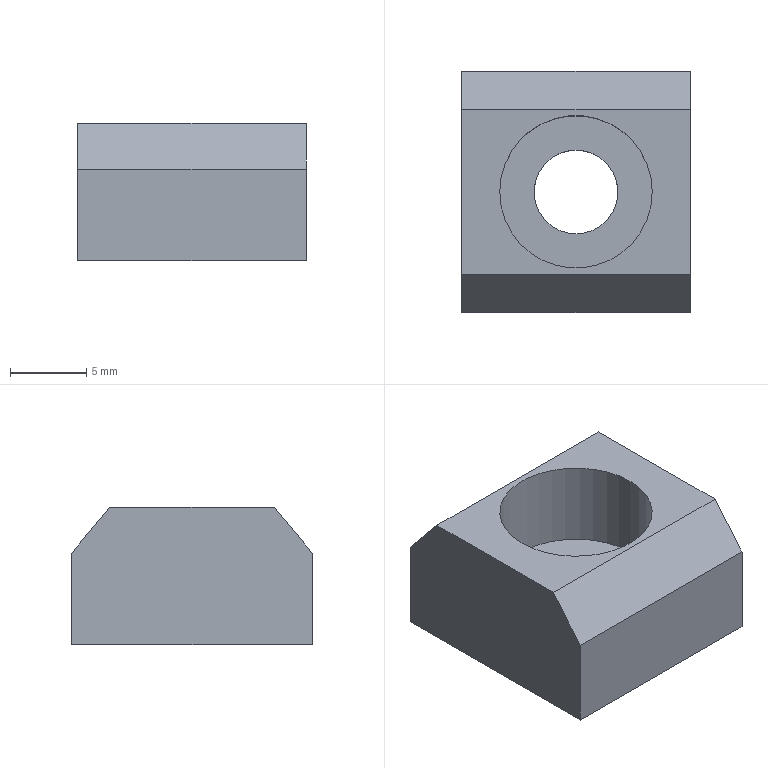Part | SolidWorks | features Extrusion 1, HoleWzd 1, ICE 1 | 1 solid | 13 faces | box 15 x 15.8 x 9 mm | volume 1494 mm3 | plane 9 | cylinder 4 | commonest cylinder face diameters 5.5 x2 10 x2
STEP:
#1=CARTESIAN_POINT('',(-5.,0.,-1.2));
#2=VERTEX_POINT('',#1);
#3=CARTESIAN_POINT('',(5.,0.,-1.2));
#4=VERTEX_POINT('',#3);
#5=CARTESIAN_POINT('',(0.,0.,-1.2));
#6=DIRECTION('',(0.,0.,1.));
#7=DIRECTION('',(1.,0.,0.));
#8=AXIS2_PLACEMENT_3D('',#5,#6,#7);
#9=CIRCLE('',#8,5.);
#10=EDGE_CURVE('',#2,#4,#9,.T.);
#11=ORIENTED_EDGE('',*,*,#10,.F.);
#12=CARTESIAN_POINT('',(-5.,0.,4.5));
#13=VERTEX_POINT('',#12);
#14=CARTESIAN_POINT('',(-5.,0.,4.5));
#15=DIRECTION('',(0.,0.,1.));
#16=VECTOR('',#15,1000.);
#17=LINE('',#14,#16);
#18=EDGE_CURVE('',#2,#13,#17,.T.);
#19=ORIENTED_EDGE('',*,*,#18,.T.);
#20=CARTESIAN_POINT('',(5.,0.,4.5));
#21=VERTEX_POINT('',#20);
#22=CARTESIAN_POINT('',(0.,0.,4.5));
#23=DIRECTION('',(0.,0.,1.));
#24=DIRECTION('',(1.,0.,0.));
#25=AXIS2_PLACEMENT_3D('',#22,#23,#24);
#26=CIRCLE('',#25,5.);
#27=EDGE_CURVE('',#13,#21,#26,.T.);
#28=ORIENTED_EDGE('',*,*,#27,.T.);
#29=CARTESIAN_POINT('',(5.,0.,4.5));
#30=DIRECTION('',(0.,0.,1.));
#31=VECTOR('',#30,1000.);
#32=LINE('',#29,#31);
#33=EDGE_CURVE('',#4,#21,#32,.T.);
#34=ORIENTED_EDGE('',*,*,#33,.F.);
#35=EDGE_LOOP('',(#11,#19,#28,#34));
#36=FACE_OUTER_BOUND('',#35,.T.);
#37=CARTESIAN_POINT('',(0.,0.,4.5));
#38=DIRECTION('',(0.,0.,1.));
#39=DIRECTION('',(1.,0.,0.));
#40=AXIS2_PLACEMENT_3D('',#37,#38,#39);
#41=CYLINDRICAL_SURFACE('',#40,5.);
#42=ADVANCED_FACE('',(#36),#41,.F.);
#43=CARTESIAN_POINT('',(-2.75,0.,-4.5));
#44=VERTEX_POINT('',#43);
#45=CARTESIAN_POINT('',(2.75,0.,-4.5));
#46=VERTEX_POINT('',#45);
#47=CARTESIAN_POINT('',(0.,0.,-4.5));
#48=DIRECTION('',(0.,0.,1.));
#49=DIRECTION('',(1.,0.,0.));
#50=AXIS2_PLACEMENT_3D('',#47,#48,#49);
#51=CIRCLE('',#50,2.75);
#52=EDGE_CURVE('',#44,#46,#51,.T.);
#53=ORIENTED_EDGE('',*,*,#52,.F.);
#54=CARTESIAN_POINT('',(-2.75,0.,-1.2));
#55=VERTEX_POINT('',#54);
#56=CARTESIAN_POINT('',(-2.75,0.,4.5));
#57=DIRECTION('',(0.,0.,1.));
#58=VECTOR('',#57,1000.);
#59=LINE('',#56,#58);
#60=EDGE_CURVE('',#44,#55,#59,.T.);
#61=ORIENTED_EDGE('',*,*,#60,.T.);
#62=CARTESIAN_POINT('',(2.75,0.,-1.2));
#63=VERTEX_POINT('',#62);
#64=CARTESIAN_POINT('',(0.,0.,-1.2));
#65=DIRECTION('',(0.,0.,1.));
#66=DIRECTION('',(1.,0.,0.));
#67=AXIS2_PLACEMENT_3D('',#64,#65,#66);
#68=CIRCLE('',#67,2.75);
#69=EDGE_CURVE('',#55,#63,#68,.T.);
#70=ORIENTED_EDGE('',*,*,#69,.T.);
#71=CARTESIAN_POINT('',(2.75,0.,4.5));
#72=DIRECTION('',(0.,0.,1.));
#73=VECTOR('',#72,1000.);
#74=LINE('',#71,#73);
#75=EDGE_CURVE('',#46,#63,#74,.T.);
#76=ORIENTED_EDGE('',*,*,#75,.F.);
#77=EDGE_LOOP('',(#53,#61,#70,#76));
#78=FACE_OUTER_BOUND('',#77,.T.);
#79=CARTESIAN_POINT('',(0.,0.,4.5));
#80=DIRECTION('',(0.,0.,1.));
#81=DIRECTION('',(1.,0.,0.));
#82=AXIS2_PLACEMENT_3D('',#79,#80,#81);
#83=CYLINDRICAL_SURFACE('',#82,2.75);
#84=ADVANCED_FACE('',(#78),#83,.F.);
#85=CARTESIAN_POINT('',(7.5,-5.4,4.5));
#86=VERTEX_POINT('',#85);
#87=CARTESIAN_POINT('',(7.5,5.4,4.5));
#88=VERTEX_POINT('',#87);
#89=CARTESIAN_POINT('',(7.5,7.9,4.5));
#90=DIRECTION('',(0.,1.,0.));
#91=VECTOR('',#90,1000.);
#92=LINE('',#89,#91);
#93=EDGE_CURVE('',#86,#88,#92,.T.);
#94=ORIENTED_EDGE('',*,*,#93,.F.);
#95=CARTESIAN_POINT('',(7.5,-7.9,1.5));
#96=VERTEX_POINT('',#95);
#97=CARTESIAN_POINT('',(7.5,-5.4,4.5));
#98=DIRECTION('',(0.,0.6402,0.7682));
#99=VECTOR('',#98,1000.);
#100=LINE('',#97,#99);
#101=EDGE_CURVE('',#96,#86,#100,.T.);
#102=ORIENTED_EDGE('',*,*,#101,.F.);
#103=CARTESIAN_POINT('',(7.5,-7.9,-4.5));
#104=VERTEX_POINT('',#103);
#105=CARTESIAN_POINT('',(7.5,-7.9,4.5));
#106=DIRECTION('',(0.,0.,-1.));
#107=VECTOR('',#106,1000.);
#108=LINE('',#105,#107);
#109=EDGE_CURVE('',#96,#104,#108,.T.);
#110=ORIENTED_EDGE('',*,*,#109,.T.);
#111=CARTESIAN_POINT('',(7.5,7.9,-4.5));
#112=VERTEX_POINT('',#111);
#113=CARTESIAN_POINT('',(7.5,7.9,-4.5));
#114=DIRECTION('',(0.,1.,0.));
#115=VECTOR('',#114,1000.);
#116=LINE('',#113,#115);
#117=EDGE_CURVE('',#104,#112,#116,.T.);
#118=ORIENTED_EDGE('',*,*,#117,.T.);
#119=CARTESIAN_POINT('',(7.5,7.9,1.5));
#120=VERTEX_POINT('',#119);
#121=CARTESIAN_POINT('',(7.5,7.9,4.5));
#122=DIRECTION('',(0.,0.,-1.));
#123=VECTOR('',#122,1000.);
#124=LINE('',#121,#123);
#125=EDGE_CURVE('',#120,#112,#124,.T.);
#126=ORIENTED_EDGE('',*,*,#125,.F.);
#127=CARTESIAN_POINT('',(7.5,7.9,1.5));
#128=DIRECTION('',(0.,0.6402,-0.7682));
#129=VECTOR('',#128,1000.);
#130=LINE('',#127,#129);
#131=EDGE_CURVE('',#88,#120,#130,.T.);
#132=ORIENTED_EDGE('',*,*,#131,.F.);
#133=EDGE_LOOP('',(#94,#102,#110,#118,#126,#132));
#134=FACE_OUTER_BOUND('',#133,.T.);
#135=CARTESIAN_POINT('',(7.5,7.9,4.5));
#136=DIRECTION('',(-1.,0.,0.));
#137=DIRECTION('',(0.,-1.,0.));
#138=AXIS2_PLACEMENT_3D('',#135,#136,#137);
#139=PLANE('',#138);
#140=ADVANCED_FACE('',(#134),#139,.F.);
#141=CARTESIAN_POINT('',(-7.5,7.9,1.5));
#142=VERTEX_POINT('',#141);
#143=CARTESIAN_POINT('',(-7.5,7.9,-4.5));
#144=VERTEX_POINT('',#143);
#145=CARTESIAN_POINT('',(-7.5,7.9,4.5));
#146=DIRECTION('',(0.,0.,-1.));
#147=VECTOR('',#146,1000.);
#148=LINE('',#145,#147);
#149=EDGE_CURVE('',#142,#144,#148,.T.);
#150=ORIENTED_EDGE('',*,*,#149,.F.);
#151=CARTESIAN_POINT('',(-7.5,7.9,1.5));
#152=DIRECTION('',(1.,0.,0.));
#153=VECTOR('',#152,1000.);
#154=LINE('',#151,#153);
#155=EDGE_CURVE('',#142,#120,#154,.T.);
#156=ORIENTED_EDGE('',*,*,#155,.T.);
#157=ORIENTED_EDGE('',*,*,#125,.T.);
#158=CARTESIAN_POINT('',(-7.5,7.9,-4.5));
#159=DIRECTION('',(-1.,0.,0.));
#160=VECTOR('',#159,1000.);
#161=LINE('',#158,#160);
#162=EDGE_CURVE('',#112,#144,#161,.T.);
#163=ORIENTED_EDGE('',*,*,#162,.T.);
#164=EDGE_LOOP('',(#150,#156,#157,#163));
#165=FACE_OUTER_BOUND('',#164,.T.);
#166=CARTESIAN_POINT('',(-7.5,7.9,4.5));
#167=DIRECTION('',(0.,-1.,0.));
#168=DIRECTION('',(0.,0.,-1.));
#169=AXIS2_PLACEMENT_3D('',#166,#167,#168);
#170=PLANE('',#169);
#171=ADVANCED_FACE('',(#165),#170,.F.);
#172=CARTESIAN_POINT('',(-7.5,-7.9,1.5));
#173=VERTEX_POINT('',#172);
#174=CARTESIAN_POINT('',(-7.5,-7.9,-4.5));
#175=VERTEX_POINT('',#174);
#176=CARTESIAN_POINT('',(-7.5,-7.9,4.5));
#177=DIRECTION('',(0.,0.,-1.));
#178=VECTOR('',#177,1000.);
#179=LINE('',#176,#178);
#180=EDGE_CURVE('',#173,#175,#179,.T.);
#181=ORIENTED_EDGE('',*,*,#180,.F.);
#182=CARTESIAN_POINT('',(-7.5,-5.4,4.5));
#183=VERTEX_POINT('',#182);
#184=CARTESIAN_POINT('',(-7.5,-5.4,4.5));
#185=DIRECTION('',(0.,0.6402,0.7682));
#186=VECTOR('',#185,1000.);
#187=LINE('',#184,#186);
#188=EDGE_CURVE('',#173,#183,#187,.T.);
#189=ORIENTED_EDGE('',*,*,#188,.T.);
#190=CARTESIAN_POINT('',(-7.5,5.4,4.5));
#191=VERTEX_POINT('',#190);
#192=CARTESIAN_POINT('',(-7.5,7.9,4.5));
#193=DIRECTION('',(0.,-1.,0.));
#194=VECTOR('',#193,1000.);
#195=LINE('',#192,#194);
#196=EDGE_CURVE('',#191,#183,#195,.T.);
#197=ORIENTED_EDGE('',*,*,#196,.F.);
#198=CARTESIAN_POINT('',(-7.5,7.9,1.5));
#199=DIRECTION('',(0.,0.6402,-0.7682));
#200=VECTOR('',#199,1000.);
#201=LINE('',#198,#200);
#202=EDGE_CURVE('',#191,#142,#201,.T.);
#203=ORIENTED_EDGE('',*,*,#202,.T.);
#204=ORIENTED_EDGE('',*,*,#149,.T.);
#205=CARTESIAN_POINT('',(-7.5,7.9,-4.5));
#206=DIRECTION('',(0.,-1.,0.));
#207=VECTOR('',#206,1000.);
#208=LINE('',#205,#207);
#209=EDGE_CURVE('',#144,#175,#208,.T.);
#210=ORIENTED_EDGE('',*,*,#209,.T.);
#211=EDGE_LOOP('',(#181,#189,#197,#203,#204,#210));
#212=FACE_OUTER_BOUND('',#211,.T.);
#213=CARTESIAN_POINT('',(-7.5,7.9,4.5));
#214=DIRECTION('',(1.,0.,0.));
#215=DIRECTION('',(0.,1.,0.));
#216=AXIS2_PLACEMENT_3D('',#213,#214,#215);
#217=PLANE('',#216);
#218=ADVANCED_FACE('',(#212),#217,.F.);
#219=ORIENTED_EDGE('',*,*,#109,.F.);
#220=CARTESIAN_POINT('',(-7.5,-7.9,1.5));
#221=DIRECTION('',(1.,0.,0.));
#222=VECTOR('',#221,1000.);
#223=LINE('',#220,#222);
#224=EDGE_CURVE('',#173,#96,#223,.T.);
#225=ORIENTED_EDGE('',*,*,#224,.F.);
#226=ORIENTED_EDGE('',*,*,#180,.T.);
#227=CARTESIAN_POINT('',(-7.5,-7.9,-4.5));
#228=DIRECTION('',(1.,0.,0.));
#229=VECTOR('',#228,1000.);
#230=LINE('',#227,#229);
#231=EDGE_CURVE('',#175,#104,#230,.T.);
#232=ORIENTED_EDGE('',*,*,#231,.T.);
#233=EDGE_LOOP('',(#219,#225,#226,#232));
#234=FACE_OUTER_BOUND('',#233,.T.);
#235=CARTESIAN_POINT('',(-7.5,-7.9,4.5));
#236=DIRECTION('',(0.,1.,0.));
#237=DIRECTION('',(0.,0.,1.));
#238=AXIS2_PLACEMENT_3D('',#235,#236,#237);
#239=PLANE('',#238);
#240=ADVANCED_FACE('',(#234),#239,.F.);
#241=CARTESIAN_POINT('',(-7.5,-5.4,4.5));
#242=DIRECTION('',(1.,0.,0.));
#243=VECTOR('',#242,1000.);
#244=LINE('',#241,#243);
#245=EDGE_CURVE('',#183,#86,#244,.T.);
#246=ORIENTED_EDGE('',*,*,#245,.T.);
#247=ORIENTED_EDGE('',*,*,#93,.T.);
#248=CARTESIAN_POINT('',(-7.5,5.4,4.5));
#249=DIRECTION('',(1.,0.,0.));
#250=VECTOR('',#249,1000.);
#251=LINE('',#248,#250);
#252=EDGE_CURVE('',#191,#88,#251,.T.);
#253=ORIENTED_EDGE('',*,*,#252,.F.);
#254=ORIENTED_EDGE('',*,*,#196,.T.);
#255=EDGE_LOOP('',(#246,#247,#253,#254));
#256=FACE_OUTER_BOUND('',#255,.T.);
#257=CARTESIAN_POINT('',(0.,0.,4.5));
#258=DIRECTION('',(0.,0.,1.));
#259=DIRECTION('',(1.,0.,0.));
#260=AXIS2_PLACEMENT_3D('',#257,#258,#259);
#261=CIRCLE('',#260,5.);
#262=EDGE_CURVE('',#21,#13,#261,.T.);
#263=ORIENTED_EDGE('',*,*,#262,.F.);
#264=ORIENTED_EDGE('',*,*,#27,.F.);
#265=EDGE_LOOP('',(#263,#264));
#266=FACE_BOUND('',#265,.T.);
#267=CARTESIAN_POINT('',(0.,0.,4.5));
#268=DIRECTION('',(0.,0.,1.));
#269=DIRECTION('',(1.,0.,0.));
#270=AXIS2_PLACEMENT_3D('',#267,#268,#269);
#271=PLANE('',#270);
#272=ADVANCED_FACE('',(#256,#266),#271,.T.);
#273=CARTESIAN_POINT('',(0.,0.,-4.5));
#274=DIRECTION('',(0.,0.,1.));
#275=DIRECTION('',(1.,0.,0.));
#276=AXIS2_PLACEMENT_3D('',#273,#274,#275);
#277=CIRCLE('',#276,2.75);
#278=EDGE_CURVE('',#46,#44,#277,.T.);
#279=ORIENTED_EDGE('',*,*,#278,.T.);
#280=ORIENTED_EDGE('',*,*,#52,.T.);
#281=EDGE_LOOP('',(#279,#280));
#282=FACE_BOUND('',#281,.T.);
#283=ORIENTED_EDGE('',*,*,#117,.F.);
#284=ORIENTED_EDGE('',*,*,#231,.F.);
#285=ORIENTED_EDGE('',*,*,#209,.F.);
#286=ORIENTED_EDGE('',*,*,#162,.F.);
#287=EDGE_LOOP('',(#283,#284,#285,#286));
#288=FACE_OUTER_BOUND('',#287,.T.);
#289=CARTESIAN_POINT('',(0.,0.,-4.5));
#290=DIRECTION('',(0.,0.,1.));
#291=DIRECTION('',(1.,0.,0.));
#292=AXIS2_PLACEMENT_3D('',#289,#290,#291);
#293=PLANE('',#292);
#294=ADVANCED_FACE('',(#282,#288),#293,.F.);
#295=ORIENTED_EDGE('',*,*,#60,.F.);
#296=ORIENTED_EDGE('',*,*,#278,.F.);
#297=ORIENTED_EDGE('',*,*,#75,.T.);
#298=CARTESIAN_POINT('',(0.,0.,-1.2));
#299=DIRECTION('',(0.,0.,1.));
#300=DIRECTION('',(1.,0.,0.));
#301=AXIS2_PLACEMENT_3D('',#298,#299,#300);
#302=CIRCLE('',#301,2.75);
#303=EDGE_CURVE('',#63,#55,#302,.T.);
#304=ORIENTED_EDGE('',*,*,#303,.T.);
#305=EDGE_LOOP('',(#295,#296,#297,#304));
#306=FACE_OUTER_BOUND('',#305,.T.);
#307=CARTESIAN_POINT('',(0.,0.,4.5));
#308=DIRECTION('',(0.,0.,1.));
#309=DIRECTION('',(1.,0.,0.));
#310=AXIS2_PLACEMENT_3D('',#307,#308,#309);
#311=CYLINDRICAL_SURFACE('',#310,2.75);
#312=ADVANCED_FACE('',(#306),#311,.F.);
#313=ORIENTED_EDGE('',*,*,#303,.F.);
#314=ORIENTED_EDGE('',*,*,#69,.F.);
#315=EDGE_LOOP('',(#313,#314));
#316=FACE_BOUND('',#315,.T.);
#317=CARTESIAN_POINT('',(0.,0.,-1.2));
#318=DIRECTION('',(0.,0.,1.));
#319=DIRECTION('',(1.,0.,0.));
#320=AXIS2_PLACEMENT_3D('',#317,#318,#319);
#321=CIRCLE('',#320,5.);
#322=EDGE_CURVE('',#4,#2,#321,.T.);
#323=ORIENTED_EDGE('',*,*,#322,.T.);
#324=ORIENTED_EDGE('',*,*,#10,.T.);
#325=EDGE_LOOP('',(#323,#324));
#326=FACE_OUTER_BOUND('',#325,.T.);
#327=CARTESIAN_POINT('',(2.75,0.,-1.2));
#328=DIRECTION('',(0.,0.,-1.));
#329=DIRECTION('',(-1.,0.,0.));
#330=AXIS2_PLACEMENT_3D('',#327,#328,#329);
#331=PLANE('',#330);
#332=ADVANCED_FACE('',(#316,#326),#331,.F.);
#333=ORIENTED_EDGE('',*,*,#18,.F.);
#334=ORIENTED_EDGE('',*,*,#322,.F.);
#335=ORIENTED_EDGE('',*,*,#33,.T.);
#336=ORIENTED_EDGE('',*,*,#262,.T.);
#337=EDGE_LOOP('',(#333,#334,#335,#336));
#338=FACE_OUTER_BOUND('',#337,.T.);
#339=CARTESIAN_POINT('',(0.,0.,4.5));
#340=DIRECTION('',(0.,0.,1.));
#341=DIRECTION('',(1.,0.,0.));
#342=AXIS2_PLACEMENT_3D('',#339,#340,#341);
#343=CYLINDRICAL_SURFACE('',#342,5.);
#344=ADVANCED_FACE('',(#338),#343,.F.);
#345=ORIENTED_EDGE('',*,*,#131,.T.);
#346=ORIENTED_EDGE('',*,*,#155,.F.);
#347=ORIENTED_EDGE('',*,*,#202,.F.);
#348=ORIENTED_EDGE('',*,*,#252,.T.);
#349=EDGE_LOOP('',(#345,#346,#347,#348));
#350=FACE_OUTER_BOUND('',#349,.T.);
#351=CARTESIAN_POINT('',(-7.5,7.9,1.5));
#352=DIRECTION('',(0.,-0.7682,-0.6402));
#353=DIRECTION('',(0.,0.6402,-0.7682));
#354=AXIS2_PLACEMENT_3D('',#351,#352,#353);
#355=PLANE('',#354);
#356=ADVANCED_FACE('',(#350),#355,.F.);
#357=ORIENTED_EDGE('',*,*,#101,.T.);
#358=ORIENTED_EDGE('',*,*,#245,.F.);
#359=ORIENTED_EDGE('',*,*,#188,.F.);
#360=ORIENTED_EDGE('',*,*,#224,.T.);
#361=EDGE_LOOP('',(#357,#358,#359,#360));
#362=FACE_OUTER_BOUND('',#361,.T.);
#363=CARTESIAN_POINT('',(-7.5,-5.4,4.5));
#364=DIRECTION('',(0.,0.7682,-0.6402));
#365=DIRECTION('',(0.,0.6402,0.7682));
#366=AXIS2_PLACEMENT_3D('',#363,#364,#365);
#367=PLANE('',#366);
#368=ADVANCED_FACE('',(#362),#367,.F.);
#369=CLOSED_SHELL('',(#42,#84,#140,#171,#218,#240,#272,#294,#312,#332,#344,#356,#368));
#370=MANIFOLD_SOLID_BREP('',#369);
#371=CARTESIAN_POINT('',(0.,0.,0.));
#372=DIRECTION('',(0.,0.,1.));
#373=DIRECTION('',(1.,0.,0.));
#374=AXIS2_PLACEMENT_3D('',#371,#372,#373);
#375=(LENGTH_UNIT()NAMED_UNIT(*)SI_UNIT(.MILLI.,.METRE.));
#376=UNCERTAINTY_MEASURE_WITH_UNIT(LENGTH_MEASURE(0.00001),#375,'','');
#377=(NAMED_UNIT(*)PLANE_ANGLE_UNIT()SI_UNIT($,.RADIAN.));
#378=(NAMED_UNIT(*)SI_UNIT($,.STERADIAN.)SOLID_ANGLE_UNIT());
#379=(GEOMETRIC_REPRESENTATION_CONTEXT(3)GLOBAL_UNCERTAINTY_ASSIGNED_CONTEXT((#376))GLOBAL_UNIT_ASSIGNED_CONTEXT((#375,#377,#378))REPRESENTATION_CONTEXT('',''));
#380=ADVANCED_BREP_SHAPE_REPRESENTATION('',(#370,#374),#379);